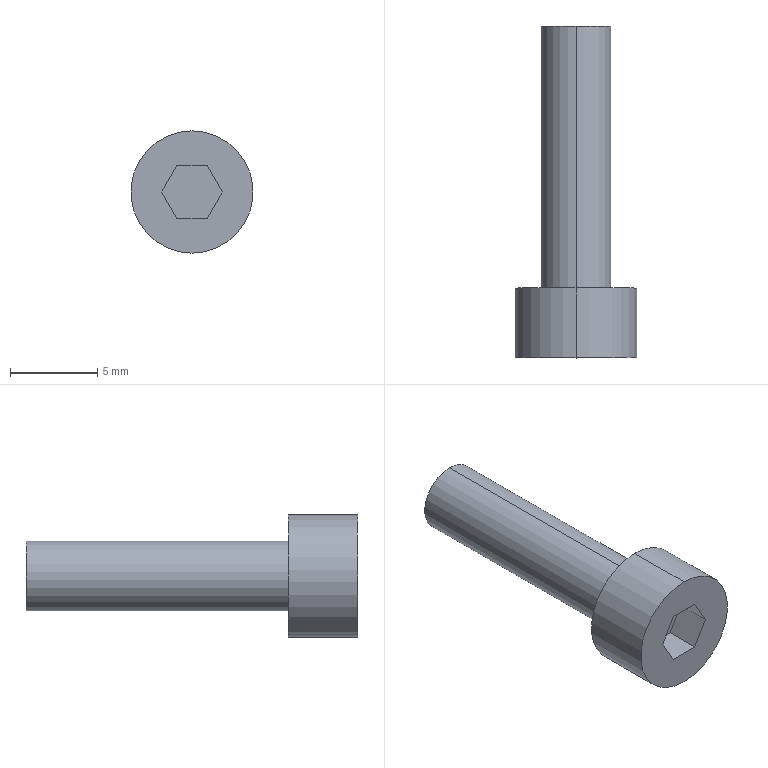Part | SolidWorks | features BaseBody 1 | 1 solid | 14 faces | box 7 x 19 x 7 mm | volume 326.845 mm3 | plane 10 | cylinder 4 | commonest cylinder face diameters 4 x2 7 x2
STEP:
#1=CARTESIAN_POINT('',(0.,19.,-2.));
#2=VERTEX_POINT('',#1);
#3=CARTESIAN_POINT('',(0.,19.,2.));
#4=VERTEX_POINT('',#3);
#5=CARTESIAN_POINT('',(0.,19.,0.));
#6=DIRECTION('',(0.,-1.,0.));
#7=DIRECTION('',(0.,0.,-1.));
#8=AXIS2_PLACEMENT_3D('',#5,#6,#7);
#9=CIRCLE('',#8,2.);
#10=EDGE_CURVE('',#2,#4,#9,.T.);
#11=ORIENTED_EDGE('',*,*,#10,.T.);
#12=CARTESIAN_POINT('',(0.,4.,2.));
#13=VERTEX_POINT('',#12);
#14=CARTESIAN_POINT('',(0.,19.,2.));
#15=DIRECTION('',(0.,-1.,0.));
#16=VECTOR('',#15,1000.);
#17=LINE('',#14,#16);
#18=EDGE_CURVE('',#4,#13,#17,.T.);
#19=ORIENTED_EDGE('',*,*,#18,.T.);
#20=CARTESIAN_POINT('',(0.,4.,-2.));
#21=VERTEX_POINT('',#20);
#22=CARTESIAN_POINT('',(0.,4.,0.));
#23=DIRECTION('',(0.,1.,0.));
#24=DIRECTION('',(0.,0.,-1.));
#25=AXIS2_PLACEMENT_3D('',#22,#23,#24);
#26=CIRCLE('',#25,2.);
#27=EDGE_CURVE('',#13,#21,#26,.T.);
#28=ORIENTED_EDGE('',*,*,#27,.T.);
#29=CARTESIAN_POINT('',(0.,19.,-2.));
#30=DIRECTION('',(0.,-1.,0.));
#31=VECTOR('',#30,1000.);
#32=LINE('',#29,#31);
#33=EDGE_CURVE('',#2,#21,#32,.T.);
#34=ORIENTED_EDGE('',*,*,#33,.F.);
#35=EDGE_LOOP('',(#11,#19,#28,#34));
#36=FACE_OUTER_BOUND('',#35,.T.);
#37=CARTESIAN_POINT('',(0.,19.,0.));
#38=DIRECTION('',(0.,-1.,0.));
#39=DIRECTION('',(0.,0.,-1.));
#40=AXIS2_PLACEMENT_3D('',#37,#38,#39);
#41=CYLINDRICAL_SURFACE('',#40,2.);
#42=ADVANCED_FACE('',(#36),#41,.T.);
#43=CARTESIAN_POINT('',(0.,4.,3.5));
#44=VERTEX_POINT('',#43);
#45=CARTESIAN_POINT('',(0.,4.,-3.5));
#46=VERTEX_POINT('',#45);
#47=CARTESIAN_POINT('',(0.,4.,0.));
#48=DIRECTION('',(0.,1.,0.));
#49=DIRECTION('',(0.,0.,-1.));
#50=AXIS2_PLACEMENT_3D('',#47,#48,#49);
#51=CIRCLE('',#50,3.5);
#52=EDGE_CURVE('',#44,#46,#51,.T.);
#53=ORIENTED_EDGE('',*,*,#52,.F.);
#54=CARTESIAN_POINT('',(0.,0.,3.5));
#55=VERTEX_POINT('',#54);
#56=CARTESIAN_POINT('',(0.,4.,3.5));
#57=DIRECTION('',(0.,-1.,0.));
#58=VECTOR('',#57,1000.);
#59=LINE('',#56,#58);
#60=EDGE_CURVE('',#44,#55,#59,.T.);
#61=ORIENTED_EDGE('',*,*,#60,.T.);
#62=CARTESIAN_POINT('',(0.,0.,-3.5));
#63=VERTEX_POINT('',#62);
#64=CARTESIAN_POINT('',(0.,0.,0.));
#65=DIRECTION('',(0.,1.,0.));
#66=DIRECTION('',(0.,0.,-1.));
#67=AXIS2_PLACEMENT_3D('',#64,#65,#66);
#68=CIRCLE('',#67,3.5);
#69=EDGE_CURVE('',#55,#63,#68,.T.);
#70=ORIENTED_EDGE('',*,*,#69,.T.);
#71=CARTESIAN_POINT('',(0.,4.,-3.5));
#72=DIRECTION('',(0.,-1.,0.));
#73=VECTOR('',#72,1000.);
#74=LINE('',#71,#73);
#75=EDGE_CURVE('',#46,#63,#74,.T.);
#76=ORIENTED_EDGE('',*,*,#75,.F.);
#77=EDGE_LOOP('',(#53,#61,#70,#76));
#78=FACE_OUTER_BOUND('',#77,.T.);
#79=CARTESIAN_POINT('',(0.,4.,0.));
#80=DIRECTION('',(0.,-1.,0.));
#81=DIRECTION('',(0.,0.,-1.));
#82=AXIS2_PLACEMENT_3D('',#79,#80,#81);
#83=CYLINDRICAL_SURFACE('',#82,3.5);
#84=ADVANCED_FACE('',(#78),#83,.T.);
#85=ORIENTED_EDGE('',*,*,#18,.F.);
#86=CARTESIAN_POINT('',(0.,19.,0.));
#87=DIRECTION('',(0.,-1.,0.));
#88=DIRECTION('',(0.,0.,-1.));
#89=AXIS2_PLACEMENT_3D('',#86,#87,#88);
#90=CIRCLE('',#89,2.);
#91=EDGE_CURVE('',#4,#2,#90,.T.);
#92=ORIENTED_EDGE('',*,*,#91,.T.);
#93=ORIENTED_EDGE('',*,*,#33,.T.);
#94=CARTESIAN_POINT('',(0.,4.,0.));
#95=DIRECTION('',(0.,1.,0.));
#96=DIRECTION('',(0.,0.,-1.));
#97=AXIS2_PLACEMENT_3D('',#94,#95,#96);
#98=CIRCLE('',#97,2.);
#99=EDGE_CURVE('',#21,#13,#98,.T.);
#100=ORIENTED_EDGE('',*,*,#99,.T.);
#101=EDGE_LOOP('',(#85,#92,#93,#100));
#102=FACE_OUTER_BOUND('',#101,.T.);
#103=CARTESIAN_POINT('',(0.,19.,0.));
#104=DIRECTION('',(0.,-1.,0.));
#105=DIRECTION('',(0.,0.,-1.));
#106=AXIS2_PLACEMENT_3D('',#103,#104,#105);
#107=CYLINDRICAL_SURFACE('',#106,2.);
#108=ADVANCED_FACE('',(#102),#107,.T.);
#109=CARTESIAN_POINT('',(0.,4.,0.));
#110=DIRECTION('',(0.,1.,0.));
#111=DIRECTION('',(0.,0.,-1.));
#112=AXIS2_PLACEMENT_3D('',#109,#110,#111);
#113=CIRCLE('',#112,3.5);
#114=EDGE_CURVE('',#46,#44,#113,.T.);
#115=ORIENTED_EDGE('',*,*,#114,.T.);
#116=ORIENTED_EDGE('',*,*,#52,.T.);
#117=EDGE_LOOP('',(#115,#116));
#118=FACE_OUTER_BOUND('',#117,.T.);
#119=ORIENTED_EDGE('',*,*,#99,.F.);
#120=ORIENTED_EDGE('',*,*,#27,.F.);
#121=EDGE_LOOP('',(#119,#120));
#122=FACE_BOUND('',#121,.T.);
#123=CARTESIAN_POINT('',(0.,4.,0.));
#124=DIRECTION('',(0.,1.,0.));
#125=DIRECTION('',(0.,0.,1.));
#126=AXIS2_PLACEMENT_3D('',#123,#124,#125);
#127=PLANE('',#126);
#128=ADVANCED_FACE('',(#118,#122),#127,.T.);
#129=ORIENTED_EDGE('',*,*,#10,.F.);
#130=ORIENTED_EDGE('',*,*,#91,.F.);
#131=EDGE_LOOP('',(#129,#130));
#132=FACE_OUTER_BOUND('',#131,.T.);
#133=CARTESIAN_POINT('',(0.,19.,0.));
#134=DIRECTION('',(0.,1.,0.));
#135=DIRECTION('',(0.,0.,1.));
#136=AXIS2_PLACEMENT_3D('',#133,#134,#135);
#137=PLANE('',#136);
#138=ADVANCED_FACE('',(#132),#137,.T.);
#139=ORIENTED_EDGE('',*,*,#60,.F.);
#140=ORIENTED_EDGE('',*,*,#114,.F.);
#141=ORIENTED_EDGE('',*,*,#75,.T.);
#142=CARTESIAN_POINT('',(0.,0.,0.));
#143=DIRECTION('',(0.,1.,0.));
#144=DIRECTION('',(0.,0.,-1.));
#145=AXIS2_PLACEMENT_3D('',#142,#143,#144);
#146=CIRCLE('',#145,3.5);
#147=EDGE_CURVE('',#63,#55,#146,.T.);
#148=ORIENTED_EDGE('',*,*,#147,.T.);
#149=EDGE_LOOP('',(#139,#140,#141,#148));
#150=FACE_OUTER_BOUND('',#149,.T.);
#151=CARTESIAN_POINT('',(0.,4.,0.));
#152=DIRECTION('',(0.,-1.,0.));
#153=DIRECTION('',(0.,0.,-1.));
#154=AXIS2_PLACEMENT_3D('',#151,#152,#153);
#155=CYLINDRICAL_SURFACE('',#154,3.5);
#156=ADVANCED_FACE('',(#150),#155,.T.);
#157=ORIENTED_EDGE('',*,*,#147,.F.);
#158=ORIENTED_EDGE('',*,*,#69,.F.);
#159=EDGE_LOOP('',(#157,#158));
#160=FACE_OUTER_BOUND('',#159,.T.);
#161=CARTESIAN_POINT('',(1.732,0.,0.));
#162=VERTEX_POINT('',#161);
#163=CARTESIAN_POINT('',(0.866,0.,-1.5));
#164=VERTEX_POINT('',#163);
#165=CARTESIAN_POINT('',(0.866,0.,-1.5));
#166=DIRECTION('',(-0.5,0.,-0.866));
#167=VECTOR('',#166,1000.);
#168=LINE('',#165,#167);
#169=EDGE_CURVE('',#162,#164,#168,.T.);
#170=ORIENTED_EDGE('',*,*,#169,.T.);
#171=CARTESIAN_POINT('',(-0.866,0.,-1.5));
#172=VERTEX_POINT('',#171);
#173=CARTESIAN_POINT('',(-0.866,0.,-1.5));
#174=DIRECTION('',(-1.,0.,0.));
#175=VECTOR('',#174,1000.);
#176=LINE('',#173,#175);
#177=EDGE_CURVE('',#164,#172,#176,.T.);
#178=ORIENTED_EDGE('',*,*,#177,.T.);
#179=CARTESIAN_POINT('',(-1.732,0.,0.));
#180=VERTEX_POINT('',#179);
#181=CARTESIAN_POINT('',(-1.732,0.,0.));
#182=DIRECTION('',(-0.5,0.,0.866));
#183=VECTOR('',#182,1000.);
#184=LINE('',#181,#183);
#185=EDGE_CURVE('',#172,#180,#184,.T.);
#186=ORIENTED_EDGE('',*,*,#185,.T.);
#187=CARTESIAN_POINT('',(-0.866,0.,1.5));
#188=VERTEX_POINT('',#187);
#189=CARTESIAN_POINT('',(-0.866,0.,1.5));
#190=DIRECTION('',(0.5,0.,0.866));
#191=VECTOR('',#190,1000.);
#192=LINE('',#189,#191);
#193=EDGE_CURVE('',#180,#188,#192,.T.);
#194=ORIENTED_EDGE('',*,*,#193,.T.);
#195=CARTESIAN_POINT('',(0.866,0.,1.5));
#196=VERTEX_POINT('',#195);
#197=CARTESIAN_POINT('',(0.866,0.,1.5));
#198=DIRECTION('',(1.,0.,0.));
#199=VECTOR('',#198,1000.);
#200=LINE('',#197,#199);
#201=EDGE_CURVE('',#188,#196,#200,.T.);
#202=ORIENTED_EDGE('',*,*,#201,.T.);
#203=CARTESIAN_POINT('',(1.732,0.,0.));
#204=DIRECTION('',(-0.5,0.,0.866));
#205=VECTOR('',#204,1000.);
#206=LINE('',#203,#205);
#207=EDGE_CURVE('',#162,#196,#206,.T.);
#208=ORIENTED_EDGE('',*,*,#207,.F.);
#209=EDGE_LOOP('',(#170,#178,#186,#194,#202,#208));
#210=FACE_BOUND('',#209,.T.);
#211=CARTESIAN_POINT('',(0.,0.,0.));
#212=DIRECTION('',(0.,1.,0.));
#213=DIRECTION('',(0.,0.,1.));
#214=AXIS2_PLACEMENT_3D('',#211,#212,#213);
#215=PLANE('',#214);
#216=ADVANCED_FACE('',(#160,#210),#215,.F.);
#217=CARTESIAN_POINT('',(0.866,2.,1.5));
#218=VERTEX_POINT('',#217);
#219=CARTESIAN_POINT('',(0.866,2.,1.5));
#220=DIRECTION('',(0.,-1.,0.));
#221=VECTOR('',#220,1000.);
#222=LINE('',#219,#221);
#223=EDGE_CURVE('',#218,#196,#222,.T.);
#224=ORIENTED_EDGE('',*,*,#223,.F.);
#225=CARTESIAN_POINT('',(1.732,2.,0.));
#226=VERTEX_POINT('',#225);
#227=CARTESIAN_POINT('',(1.732,2.,0.));
#228=DIRECTION('',(-0.5,0.,0.866));
#229=VECTOR('',#228,1000.);
#230=LINE('',#227,#229);
#231=EDGE_CURVE('',#226,#218,#230,.T.);
#232=ORIENTED_EDGE('',*,*,#231,.F.);
#233=CARTESIAN_POINT('',(1.732,2.,0.));
#234=DIRECTION('',(0.,1.,0.));
#235=VECTOR('',#234,1000.);
#236=LINE('',#233,#235);
#237=EDGE_CURVE('',#162,#226,#236,.T.);
#238=ORIENTED_EDGE('',*,*,#237,.F.);
#239=ORIENTED_EDGE('',*,*,#207,.T.);
#240=EDGE_LOOP('',(#224,#232,#238,#239));
#241=FACE_OUTER_BOUND('',#240,.T.);
#242=CARTESIAN_POINT('',(1.732,2.,0.));
#243=DIRECTION('',(0.866,0.,0.5));
#244=DIRECTION('',(0.5,0.,-0.866));
#245=AXIS2_PLACEMENT_3D('',#242,#243,#244);
#246=PLANE('',#245);
#247=ADVANCED_FACE('',(#241),#246,.F.);
#248=CARTESIAN_POINT('',(-0.866,2.,1.5));
#249=VERTEX_POINT('',#248);
#250=CARTESIAN_POINT('',(-0.866,2.,1.5));
#251=DIRECTION('',(0.,-1.,0.));
#252=VECTOR('',#251,1000.);
#253=LINE('',#250,#252);
#254=EDGE_CURVE('',#249,#188,#253,.T.);
#255=ORIENTED_EDGE('',*,*,#254,.F.);
#256=CARTESIAN_POINT('',(0.866,2.,1.5));
#257=DIRECTION('',(-1.,0.,0.));
#258=VECTOR('',#257,1000.);
#259=LINE('',#256,#258);
#260=EDGE_CURVE('',#218,#249,#259,.T.);
#261=ORIENTED_EDGE('',*,*,#260,.F.);
#262=ORIENTED_EDGE('',*,*,#223,.T.);
#263=ORIENTED_EDGE('',*,*,#201,.F.);
#264=EDGE_LOOP('',(#255,#261,#262,#263));
#265=FACE_OUTER_BOUND('',#264,.T.);
#266=CARTESIAN_POINT('',(0.866,2.,1.5));
#267=DIRECTION('',(0.,0.,1.));
#268=DIRECTION('',(1.,0.,0.));
#269=AXIS2_PLACEMENT_3D('',#266,#267,#268);
#270=PLANE('',#269);
#271=ADVANCED_FACE('',(#265),#270,.F.);
#272=CARTESIAN_POINT('',(-1.732,2.,0.));
#273=VERTEX_POINT('',#272);
#274=CARTESIAN_POINT('',(-0.866,2.,-1.5));
#275=VERTEX_POINT('',#274);
#276=CARTESIAN_POINT('',(-1.732,2.,0.));
#277=DIRECTION('',(0.5,0.,-0.866));
#278=VECTOR('',#277,1000.);
#279=LINE('',#276,#278);
#280=EDGE_CURVE('',#273,#275,#279,.T.);
#281=ORIENTED_EDGE('',*,*,#280,.T.);
#282=CARTESIAN_POINT('',(0.866,2.,-1.5));
#283=VERTEX_POINT('',#282);
#284=CARTESIAN_POINT('',(-0.866,2.,-1.5));
#285=DIRECTION('',(1.,0.,0.));
#286=VECTOR('',#285,1000.);
#287=LINE('',#284,#286);
#288=EDGE_CURVE('',#275,#283,#287,.T.);
#289=ORIENTED_EDGE('',*,*,#288,.T.);
#290=CARTESIAN_POINT('',(0.866,2.,-1.5));
#291=DIRECTION('',(0.5,0.,0.866));
#292=VECTOR('',#291,1000.);
#293=LINE('',#290,#292);
#294=EDGE_CURVE('',#283,#226,#293,.T.);
#295=ORIENTED_EDGE('',*,*,#294,.T.);
#296=ORIENTED_EDGE('',*,*,#231,.T.);
#297=ORIENTED_EDGE('',*,*,#260,.T.);
#298=CARTESIAN_POINT('',(-0.866,2.,1.5));
#299=DIRECTION('',(-0.5,0.,-0.866));
#300=VECTOR('',#299,1000.);
#301=LINE('',#298,#300);
#302=EDGE_CURVE('',#249,#273,#301,.T.);
#303=ORIENTED_EDGE('',*,*,#302,.T.);
#304=EDGE_LOOP('',(#281,#289,#295,#296,#297,#303));
#305=FACE_OUTER_BOUND('',#304,.T.);
#306=CARTESIAN_POINT('',(0.,2.,0.));
#307=DIRECTION('',(0.,-1.,0.));
#308=DIRECTION('',(0.,0.,-1.));
#309=AXIS2_PLACEMENT_3D('',#306,#307,#308);
#310=PLANE('',#309);
#311=ADVANCED_FACE('',(#305),#310,.T.);
#312=ORIENTED_EDGE('',*,*,#237,.T.);
#313=ORIENTED_EDGE('',*,*,#294,.F.);
#314=CARTESIAN_POINT('',(0.866,2.,-1.5));
#315=DIRECTION('',(0.,1.,0.));
#316=VECTOR('',#315,1000.);
#317=LINE('',#314,#316);
#318=EDGE_CURVE('',#164,#283,#317,.T.);
#319=ORIENTED_EDGE('',*,*,#318,.F.);
#320=ORIENTED_EDGE('',*,*,#169,.F.);
#321=EDGE_LOOP('',(#312,#313,#319,#320));
#322=FACE_OUTER_BOUND('',#321,.T.);
#323=CARTESIAN_POINT('',(0.866,2.,-1.5));
#324=DIRECTION('',(0.866,0.,-0.5));
#325=DIRECTION('',(-0.5,0.,-0.866));
#326=AXIS2_PLACEMENT_3D('',#323,#324,#325);
#327=PLANE('',#326);
#328=ADVANCED_FACE('',(#322),#327,.F.);
#329=CARTESIAN_POINT('',(-1.732,2.,0.));
#330=DIRECTION('',(0.,-1.,0.));
#331=VECTOR('',#330,1000.);
#332=LINE('',#329,#331);
#333=EDGE_CURVE('',#273,#180,#332,.T.);
#334=ORIENTED_EDGE('',*,*,#333,.F.);
#335=ORIENTED_EDGE('',*,*,#302,.F.);
#336=ORIENTED_EDGE('',*,*,#254,.T.);
#337=ORIENTED_EDGE('',*,*,#193,.F.);
#338=EDGE_LOOP('',(#334,#335,#336,#337));
#339=FACE_OUTER_BOUND('',#338,.T.);
#340=CARTESIAN_POINT('',(-0.866,2.,1.5));
#341=DIRECTION('',(-0.866,0.,0.5));
#342=DIRECTION('',(0.5,0.,0.866));
#343=AXIS2_PLACEMENT_3D('',#340,#341,#342);
#344=PLANE('',#343);
#345=ADVANCED_FACE('',(#339),#344,.F.);
#346=ORIENTED_EDGE('',*,*,#318,.T.);
#347=ORIENTED_EDGE('',*,*,#288,.F.);
#348=CARTESIAN_POINT('',(-0.866,2.,-1.5));
#349=DIRECTION('',(0.,1.,0.));
#350=VECTOR('',#349,1000.);
#351=LINE('',#348,#350);
#352=EDGE_CURVE('',#172,#275,#351,.T.);
#353=ORIENTED_EDGE('',*,*,#352,.F.);
#354=ORIENTED_EDGE('',*,*,#177,.F.);
#355=EDGE_LOOP('',(#346,#347,#353,#354));
#356=FACE_OUTER_BOUND('',#355,.T.);
#357=CARTESIAN_POINT('',(-0.866,2.,-1.5));
#358=DIRECTION('',(0.,0.,-1.));
#359=DIRECTION('',(-1.,0.,0.));
#360=AXIS2_PLACEMENT_3D('',#357,#358,#359);
#361=PLANE('',#360);
#362=ADVANCED_FACE('',(#356),#361,.F.);
#363=ORIENTED_EDGE('',*,*,#352,.T.);
#364=ORIENTED_EDGE('',*,*,#280,.F.);
#365=ORIENTED_EDGE('',*,*,#333,.T.);
#366=ORIENTED_EDGE('',*,*,#185,.F.);
#367=EDGE_LOOP('',(#363,#364,#365,#366));
#368=FACE_OUTER_BOUND('',#367,.T.);
#369=CARTESIAN_POINT('',(-1.732,2.,0.));
#370=DIRECTION('',(-0.866,0.,-0.5));
#371=DIRECTION('',(-0.5,0.,0.866));
#372=AXIS2_PLACEMENT_3D('',#369,#370,#371);
#373=PLANE('',#372);
#374=ADVANCED_FACE('',(#368),#373,.F.);
#375=CLOSED_SHELL('',(#42,#84,#108,#128,#138,#156,#216,#247,#271,#311,#328,#345,#362,#374));
#376=MANIFOLD_SOLID_BREP('',#375);
#377=CARTESIAN_POINT('',(0.,0.,0.));
#378=DIRECTION('',(0.,0.,1.));
#379=DIRECTION('',(1.,0.,0.));
#380=AXIS2_PLACEMENT_3D('',#377,#378,#379);
#381=(LENGTH_UNIT()NAMED_UNIT(*)SI_UNIT(.MILLI.,.METRE.));
#382=UNCERTAINTY_MEASURE_WITH_UNIT(LENGTH_MEASURE(0.00001),#381,'','');
#383=(NAMED_UNIT(*)PLANE_ANGLE_UNIT()SI_UNIT($,.RADIAN.));
#384=(NAMED_UNIT(*)SI_UNIT($,.STERADIAN.)SOLID_ANGLE_UNIT());
#385=(GEOMETRIC_REPRESENTATION_CONTEXT(3)GLOBAL_UNCERTAINTY_ASSIGNED_CONTEXT((#382))GLOBAL_UNIT_ASSIGNED_CONTEXT((#381,#383,#384))REPRESENTATION_CONTEXT('',''));
#386=ADVANCED_BREP_SHAPE_REPRESENTATION('',(#376,#380),#385);